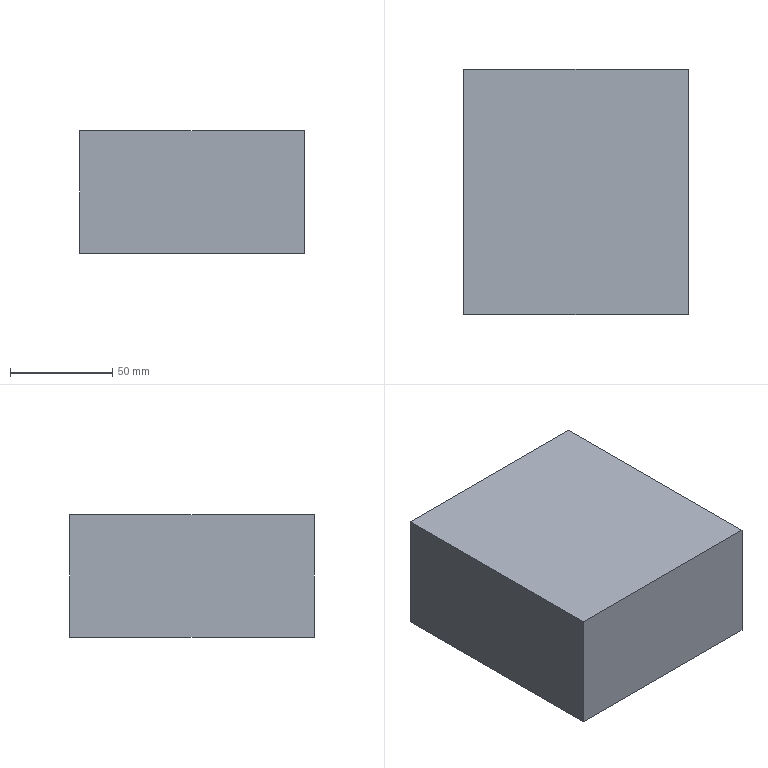Part | SolidWorks | features Extrusion 1, HoleWzd 1, PLine 1 | 1 solid | 15 faces | box 110 x 120 x 60 mm | volume 791822 mm3 | plane 7 | cylinder 4 | cone 4 | commonest cylinder face diameters 3.3 x4
STEP:
#1=CARTESIAN_POINT('',(1.65,15.,-19.9));
#2=VERTEX_POINT('',#1);
#3=CARTESIAN_POINT('',(-1.65,15.,-19.9));
#4=VERTEX_POINT('',#3);
#5=CARTESIAN_POINT('',(0.,15.,-19.9));
#6=DIRECTION('',(0.,0.,-1.));
#7=DIRECTION('',(-1.,0.,0.));
#8=AXIS2_PLACEMENT_3D('',#5,#6,#7);
#9=CIRCLE('',#8,1.65);
#10=EDGE_CURVE('',#2,#4,#9,.T.);
#11=ORIENTED_EDGE('',*,*,#10,.F.);
#12=CARTESIAN_POINT('',(1.65,15.,-30.));
#13=VERTEX_POINT('',#12);
#14=CARTESIAN_POINT('',(1.65,15.,-30.));
#15=DIRECTION('',(0.,0.,-1.));
#16=VECTOR('',#15,1000.);
#17=LINE('',#14,#16);
#18=EDGE_CURVE('',#2,#13,#17,.T.);
#19=ORIENTED_EDGE('',*,*,#18,.T.);
#20=CARTESIAN_POINT('',(-1.65,15.,-30.));
#21=VERTEX_POINT('',#20);
#22=CARTESIAN_POINT('',(0.,15.,-30.));
#23=DIRECTION('',(0.,0.,-1.));
#24=DIRECTION('',(-1.,0.,0.));
#25=AXIS2_PLACEMENT_3D('',#22,#23,#24);
#26=CIRCLE('',#25,1.65);
#27=EDGE_CURVE('',#13,#21,#26,.T.);
#28=ORIENTED_EDGE('',*,*,#27,.T.);
#29=CARTESIAN_POINT('',(-1.65,15.,-30.));
#30=DIRECTION('',(0.,0.,-1.));
#31=VECTOR('',#30,1000.);
#32=LINE('',#29,#31);
#33=EDGE_CURVE('',#4,#21,#32,.T.);
#34=ORIENTED_EDGE('',*,*,#33,.F.);
#35=EDGE_LOOP('',(#11,#19,#28,#34));
#36=FACE_OUTER_BOUND('',#35,.T.);
#37=CARTESIAN_POINT('',(0.,15.,-30.));
#38=DIRECTION('',(0.,0.,-1.));
#39=DIRECTION('',(-1.,0.,0.));
#40=AXIS2_PLACEMENT_3D('',#37,#38,#39);
#41=CYLINDRICAL_SURFACE('',#40,1.65);
#42=ADVANCED_FACE('',(#36),#41,.F.);
#43=CARTESIAN_POINT('',(0.,15.,-18.909));
#44=VERTEX_POINT('',#43);
#45=CARTESIAN_POINT('',(-1.65,15.,-19.9));
#46=DIRECTION('',(-0.8572,0.,-0.515));
#47=VECTOR('',#46,1000.);
#48=LINE('',#45,#47);
#49=EDGE_CURVE('',#44,#4,#48,.T.);
#50=ORIENTED_EDGE('',*,*,#49,.F.);
#51=CARTESIAN_POINT('',(1.65,15.,-19.9));
#52=DIRECTION('',(0.8572,0.,-0.515));
#53=VECTOR('',#52,1000.);
#54=LINE('',#51,#53);
#55=EDGE_CURVE('',#44,#2,#54,.T.);
#56=ORIENTED_EDGE('',*,*,#55,.T.);
#57=ORIENTED_EDGE('',*,*,#10,.T.);
#58=EDGE_LOOP('',(#50,#56,#57));
#59=FACE_OUTER_BOUND('',#58,.T.);
#60=CARTESIAN_POINT('',(0.,15.,-19.9));
#61=DIRECTION('',(0.,0.,-1.));
#62=DIRECTION('',(-1.,0.,0.));
#63=AXIS2_PLACEMENT_3D('',#60,#61,#62);
#64=CONICAL_SURFACE('',#63,1.65,1.03);
#65=ADVANCED_FACE('',(#59),#64,.F.);
#66=CARTESIAN_POINT('',(1.65,-15.,-19.9));
#67=VERTEX_POINT('',#66);
#68=CARTESIAN_POINT('',(-1.65,-15.,-19.9));
#69=VERTEX_POINT('',#68);
#70=CARTESIAN_POINT('',(0.,-15.,-19.9));
#71=DIRECTION('',(0.,0.,-1.));
#72=DIRECTION('',(-1.,0.,0.));
#73=AXIS2_PLACEMENT_3D('',#70,#71,#72);
#74=CIRCLE('',#73,1.65);
#75=EDGE_CURVE('',#67,#69,#74,.T.);
#76=ORIENTED_EDGE('',*,*,#75,.F.);
#77=CARTESIAN_POINT('',(1.65,-15.,-30.));
#78=VERTEX_POINT('',#77);
#79=CARTESIAN_POINT('',(1.65,-15.,-30.));
#80=DIRECTION('',(0.,0.,-1.));
#81=VECTOR('',#80,1000.);
#82=LINE('',#79,#81);
#83=EDGE_CURVE('',#67,#78,#82,.T.);
#84=ORIENTED_EDGE('',*,*,#83,.T.);
#85=CARTESIAN_POINT('',(-1.65,-15.,-30.));
#86=VERTEX_POINT('',#85);
#87=CARTESIAN_POINT('',(0.,-15.,-30.));
#88=DIRECTION('',(0.,0.,-1.));
#89=DIRECTION('',(-1.,0.,0.));
#90=AXIS2_PLACEMENT_3D('',#87,#88,#89);
#91=CIRCLE('',#90,1.65);
#92=EDGE_CURVE('',#78,#86,#91,.T.);
#93=ORIENTED_EDGE('',*,*,#92,.T.);
#94=CARTESIAN_POINT('',(-1.65,-15.,-30.));
#95=DIRECTION('',(0.,0.,-1.));
#96=VECTOR('',#95,1000.);
#97=LINE('',#94,#96);
#98=EDGE_CURVE('',#69,#86,#97,.T.);
#99=ORIENTED_EDGE('',*,*,#98,.F.);
#100=EDGE_LOOP('',(#76,#84,#93,#99));
#101=FACE_OUTER_BOUND('',#100,.T.);
#102=CARTESIAN_POINT('',(0.,-15.,-30.));
#103=DIRECTION('',(0.,0.,-1.));
#104=DIRECTION('',(-1.,0.,0.));
#105=AXIS2_PLACEMENT_3D('',#102,#103,#104);
#106=CYLINDRICAL_SURFACE('',#105,1.65);
#107=ADVANCED_FACE('',(#101),#106,.F.);
#108=CARTESIAN_POINT('',(0.,-15.,-18.909));
#109=VERTEX_POINT('',#108);
#110=CARTESIAN_POINT('',(-1.65,-15.,-19.9));
#111=DIRECTION('',(-0.8572,0.,-0.515));
#112=VECTOR('',#111,1000.);
#113=LINE('',#110,#112);
#114=EDGE_CURVE('',#109,#69,#113,.T.);
#115=ORIENTED_EDGE('',*,*,#114,.F.);
#116=CARTESIAN_POINT('',(1.65,-15.,-19.9));
#117=DIRECTION('',(0.8572,0.,-0.515));
#118=VECTOR('',#117,1000.);
#119=LINE('',#116,#118);
#120=EDGE_CURVE('',#109,#67,#119,.T.);
#121=ORIENTED_EDGE('',*,*,#120,.T.);
#122=ORIENTED_EDGE('',*,*,#75,.T.);
#123=EDGE_LOOP('',(#115,#121,#122));
#124=FACE_OUTER_BOUND('',#123,.T.);
#125=CARTESIAN_POINT('',(0.,-15.,-19.9));
#126=DIRECTION('',(0.,0.,-1.));
#127=DIRECTION('',(-1.,0.,0.));
#128=AXIS2_PLACEMENT_3D('',#125,#126,#127);
#129=CONICAL_SURFACE('',#128,1.65,1.03);
#130=ADVANCED_FACE('',(#124),#129,.F.);
#131=CARTESIAN_POINT('',(55.,-60.,-30.));
#132=VERTEX_POINT('',#131);
#133=CARTESIAN_POINT('',(55.,60.,-30.));
#134=VERTEX_POINT('',#133);
#135=CARTESIAN_POINT('',(55.,-60.,-30.));
#136=DIRECTION('',(0.,1.,0.));
#137=VECTOR('',#136,1000.);
#138=LINE('',#135,#137);
#139=EDGE_CURVE('',#132,#134,#138,.T.);
#140=ORIENTED_EDGE('',*,*,#139,.T.);
#141=CARTESIAN_POINT('',(55.,60.,30.));
#142=VERTEX_POINT('',#141);
#143=CARTESIAN_POINT('',(55.,60.,30.));
#144=DIRECTION('',(0.,0.,-1.));
#145=VECTOR('',#144,1000.);
#146=LINE('',#143,#145);
#147=EDGE_CURVE('',#142,#134,#146,.T.);
#148=ORIENTED_EDGE('',*,*,#147,.F.);
#149=CARTESIAN_POINT('',(55.,-60.,30.));
#150=VERTEX_POINT('',#149);
#151=CARTESIAN_POINT('',(55.,-60.,30.));
#152=DIRECTION('',(0.,1.,0.));
#153=VECTOR('',#152,1000.);
#154=LINE('',#151,#153);
#155=EDGE_CURVE('',#150,#142,#154,.T.);
#156=ORIENTED_EDGE('',*,*,#155,.F.);
#157=CARTESIAN_POINT('',(55.,-60.,30.));
#158=DIRECTION('',(0.,0.,-1.));
#159=VECTOR('',#158,1000.);
#160=LINE('',#157,#159);
#161=EDGE_CURVE('',#150,#132,#160,.T.);
#162=ORIENTED_EDGE('',*,*,#161,.T.);
#163=EDGE_LOOP('',(#140,#148,#156,#162));
#164=FACE_OUTER_BOUND('',#163,.T.);
#165=CARTESIAN_POINT('',(55.,-40.,-13.));
#166=VERTEX_POINT('',#165);
#167=CARTESIAN_POINT('',(55.,50.,-13.));
#168=VERTEX_POINT('',#167);
#169=CARTESIAN_POINT('',(55.,-60.,-13.));
#170=DIRECTION('',(0.,1.,0.));
#171=VECTOR('',#170,1000.);
#172=LINE('',#169,#171);
#173=EDGE_CURVE('',#166,#168,#172,.T.);
#174=ORIENTED_EDGE('',*,*,#173,.F.);
#175=CARTESIAN_POINT('',(55.,-40.,27.));
#176=VERTEX_POINT('',#175);
#177=CARTESIAN_POINT('',(55.,-40.,30.));
#178=DIRECTION('',(0.,0.,-1.));
#179=VECTOR('',#178,1000.);
#180=LINE('',#177,#179);
#181=EDGE_CURVE('',#176,#166,#180,.T.);
#182=ORIENTED_EDGE('',*,*,#181,.F.);
#183=CARTESIAN_POINT('',(55.,50.,27.));
#184=VERTEX_POINT('',#183);
#185=CARTESIAN_POINT('',(55.,-60.,27.));
#186=DIRECTION('',(0.,-1.,0.));
#187=VECTOR('',#186,1000.);
#188=LINE('',#185,#187);
#189=EDGE_CURVE('',#184,#176,#188,.T.);
#190=ORIENTED_EDGE('',*,*,#189,.F.);
#191=CARTESIAN_POINT('',(55.,50.,30.));
#192=DIRECTION('',(0.,0.,1.));
#193=VECTOR('',#192,1000.);
#194=LINE('',#191,#193);
#195=EDGE_CURVE('',#168,#184,#194,.T.);
#196=ORIENTED_EDGE('',*,*,#195,.F.);
#197=EDGE_LOOP('',(#174,#182,#190,#196));
#198=FACE_BOUND('',#197,.T.);
#199=CARTESIAN_POINT('',(55.,-60.,30.));
#200=DIRECTION('',(-1.,0.,0.));
#201=DIRECTION('',(0.,0.,1.));
#202=AXIS2_PLACEMENT_3D('',#199,#200,#201);
#203=PLANE('',#202);
#204=ADVANCED_FACE('',(#164,#198),#203,.F.);
#205=ORIENTED_EDGE('',*,*,#181,.T.);
#206=ORIENTED_EDGE('',*,*,#173,.T.);
#207=ORIENTED_EDGE('',*,*,#195,.T.);
#208=ORIENTED_EDGE('',*,*,#189,.T.);
#209=EDGE_LOOP('',(#205,#206,#207,#208));
#210=FACE_OUTER_BOUND('',#209,.T.);
#211=CARTESIAN_POINT('',(55.,-60.,30.));
#212=DIRECTION('',(-1.,0.,0.));
#213=DIRECTION('',(0.,0.,1.));
#214=AXIS2_PLACEMENT_3D('',#211,#212,#213);
#215=PLANE('',#214);
#216=ADVANCED_FACE('',(#210),#215,.F.);
#217=CARTESIAN_POINT('',(-55.,60.,-30.));
#218=VERTEX_POINT('',#217);
#219=CARTESIAN_POINT('',(-55.,60.,-30.));
#220=DIRECTION('',(-1.,0.,0.));
#221=VECTOR('',#220,1000.);
#222=LINE('',#219,#221);
#223=EDGE_CURVE('',#134,#218,#222,.T.);
#224=ORIENTED_EDGE('',*,*,#223,.T.);
#225=CARTESIAN_POINT('',(-55.,60.,30.));
#226=VERTEX_POINT('',#225);
#227=CARTESIAN_POINT('',(-55.,60.,30.));
#228=DIRECTION('',(0.,0.,-1.));
#229=VECTOR('',#228,1000.);
#230=LINE('',#227,#229);
#231=EDGE_CURVE('',#226,#218,#230,.T.);
#232=ORIENTED_EDGE('',*,*,#231,.F.);
#233=CARTESIAN_POINT('',(-55.,60.,30.));
#234=DIRECTION('',(-1.,0.,0.));
#235=VECTOR('',#234,1000.);
#236=LINE('',#233,#235);
#237=EDGE_CURVE('',#142,#226,#236,.T.);
#238=ORIENTED_EDGE('',*,*,#237,.F.);
#239=ORIENTED_EDGE('',*,*,#147,.T.);
#240=EDGE_LOOP('',(#224,#232,#238,#239));
#241=FACE_OUTER_BOUND('',#240,.T.);
#242=CARTESIAN_POINT('',(-55.,60.,30.));
#243=DIRECTION('',(0.,-1.,0.));
#244=DIRECTION('',(0.,0.,-1.));
#245=AXIS2_PLACEMENT_3D('',#242,#243,#244);
#246=PLANE('',#245);
#247=ADVANCED_FACE('',(#241),#246,.F.);
#248=CARTESIAN_POINT('',(-55.,-60.,-30.));
#249=VERTEX_POINT('',#248);
#250=CARTESIAN_POINT('',(-55.,-60.,-30.));
#251=DIRECTION('',(0.,-1.,0.));
#252=VECTOR('',#251,1000.);
#253=LINE('',#250,#252);
#254=EDGE_CURVE('',#218,#249,#253,.T.);
#255=ORIENTED_EDGE('',*,*,#254,.T.);
#256=CARTESIAN_POINT('',(-55.,-60.,30.));
#257=VERTEX_POINT('',#256);
#258=CARTESIAN_POINT('',(-55.,-60.,30.));
#259=DIRECTION('',(0.,0.,-1.));
#260=VECTOR('',#259,1000.);
#261=LINE('',#258,#260);
#262=EDGE_CURVE('',#257,#249,#261,.T.);
#263=ORIENTED_EDGE('',*,*,#262,.F.);
#264=CARTESIAN_POINT('',(-55.,-60.,30.));
#265=DIRECTION('',(0.,-1.,0.));
#266=VECTOR('',#265,1000.);
#267=LINE('',#264,#266);
#268=EDGE_CURVE('',#226,#257,#267,.T.);
#269=ORIENTED_EDGE('',*,*,#268,.F.);
#270=ORIENTED_EDGE('',*,*,#231,.T.);
#271=EDGE_LOOP('',(#255,#263,#269,#270));
#272=FACE_OUTER_BOUND('',#271,.T.);
#273=CARTESIAN_POINT('',(-55.,-60.,30.));
#274=DIRECTION('',(1.,0.,0.));
#275=DIRECTION('',(0.,0.,-1.));
#276=AXIS2_PLACEMENT_3D('',#273,#274,#275);
#277=PLANE('',#276);
#278=ADVANCED_FACE('',(#272),#277,.F.);
#279=CARTESIAN_POINT('',(-55.,-60.,-30.));
#280=DIRECTION('',(1.,0.,0.));
#281=VECTOR('',#280,1000.);
#282=LINE('',#279,#281);
#283=EDGE_CURVE('',#249,#132,#282,.T.);
#284=ORIENTED_EDGE('',*,*,#283,.T.);
#285=ORIENTED_EDGE('',*,*,#161,.F.);
#286=CARTESIAN_POINT('',(-55.,-60.,30.));
#287=DIRECTION('',(1.,0.,0.));
#288=VECTOR('',#287,1000.);
#289=LINE('',#286,#288);
#290=EDGE_CURVE('',#257,#150,#289,.T.);
#291=ORIENTED_EDGE('',*,*,#290,.F.);
#292=ORIENTED_EDGE('',*,*,#262,.T.);
#293=EDGE_LOOP('',(#284,#285,#291,#292));
#294=FACE_OUTER_BOUND('',#293,.T.);
#295=CARTESIAN_POINT('',(-55.,-60.,30.));
#296=DIRECTION('',(0.,1.,0.));
#297=DIRECTION('',(0.,0.,1.));
#298=AXIS2_PLACEMENT_3D('',#295,#296,#297);
#299=PLANE('',#298);
#300=ADVANCED_FACE('',(#294),#299,.F.);
#301=ORIENTED_EDGE('',*,*,#155,.T.);
#302=ORIENTED_EDGE('',*,*,#237,.T.);
#303=ORIENTED_EDGE('',*,*,#268,.T.);
#304=ORIENTED_EDGE('',*,*,#290,.T.);
#305=EDGE_LOOP('',(#301,#302,#303,#304));
#306=FACE_OUTER_BOUND('',#305,.T.);
#307=CARTESIAN_POINT('',(0.,0.,30.));
#308=DIRECTION('',(0.,0.,-1.));
#309=DIRECTION('',(-1.,0.,0.));
#310=AXIS2_PLACEMENT_3D('',#307,#308,#309);
#311=PLANE('',#310);
#312=ADVANCED_FACE('',(#306),#311,.F.);
#313=CARTESIAN_POINT('',(0.,15.,-30.));
#314=DIRECTION('',(0.,0.,-1.));
#315=DIRECTION('',(-1.,0.,0.));
#316=AXIS2_PLACEMENT_3D('',#313,#314,#315);
#317=CIRCLE('',#316,1.65);
#318=EDGE_CURVE('',#21,#13,#317,.T.);
#319=ORIENTED_EDGE('',*,*,#318,.F.);
#320=ORIENTED_EDGE('',*,*,#27,.F.);
#321=EDGE_LOOP('',(#319,#320));
#322=FACE_BOUND('',#321,.T.);
#323=CARTESIAN_POINT('',(0.,-15.,-30.));
#324=DIRECTION('',(0.,0.,-1.));
#325=DIRECTION('',(-1.,0.,0.));
#326=AXIS2_PLACEMENT_3D('',#323,#324,#325);
#327=CIRCLE('',#326,1.65);
#328=EDGE_CURVE('',#86,#78,#327,.T.);
#329=ORIENTED_EDGE('',*,*,#328,.F.);
#330=ORIENTED_EDGE('',*,*,#92,.F.);
#331=EDGE_LOOP('',(#329,#330));
#332=FACE_BOUND('',#331,.T.);
#333=ORIENTED_EDGE('',*,*,#139,.F.);
#334=ORIENTED_EDGE('',*,*,#283,.F.);
#335=ORIENTED_EDGE('',*,*,#254,.F.);
#336=ORIENTED_EDGE('',*,*,#223,.F.);
#337=EDGE_LOOP('',(#333,#334,#335,#336));
#338=FACE_OUTER_BOUND('',#337,.T.);
#339=CARTESIAN_POINT('',(0.,0.,-30.));
#340=DIRECTION('',(0.,0.,-1.));
#341=DIRECTION('',(-1.,0.,0.));
#342=AXIS2_PLACEMENT_3D('',#339,#340,#341);
#343=PLANE('',#342);
#344=ADVANCED_FACE('',(#322,#332,#338),#343,.T.);
#345=ORIENTED_EDGE('',*,*,#120,.F.);
#346=ORIENTED_EDGE('',*,*,#114,.T.);
#347=CARTESIAN_POINT('',(0.,-15.,-19.9));
#348=DIRECTION('',(0.,0.,-1.));
#349=DIRECTION('',(-1.,0.,0.));
#350=AXIS2_PLACEMENT_3D('',#347,#348,#349);
#351=CIRCLE('',#350,1.65);
#352=EDGE_CURVE('',#69,#67,#351,.T.);
#353=ORIENTED_EDGE('',*,*,#352,.T.);
#354=EDGE_LOOP('',(#345,#346,#353));
#355=FACE_OUTER_BOUND('',#354,.T.);
#356=CARTESIAN_POINT('',(0.,-15.,-19.9));
#357=DIRECTION('',(0.,0.,-1.));
#358=DIRECTION('',(-1.,0.,0.));
#359=AXIS2_PLACEMENT_3D('',#356,#357,#358);
#360=CONICAL_SURFACE('',#359,1.65,1.03);
#361=ADVANCED_FACE('',(#355),#360,.F.);
#362=ORIENTED_EDGE('',*,*,#83,.F.);
#363=ORIENTED_EDGE('',*,*,#352,.F.);
#364=ORIENTED_EDGE('',*,*,#98,.T.);
#365=ORIENTED_EDGE('',*,*,#328,.T.);
#366=EDGE_LOOP('',(#362,#363,#364,#365));
#367=FACE_OUTER_BOUND('',#366,.T.);
#368=CARTESIAN_POINT('',(0.,-15.,-30.));
#369=DIRECTION('',(0.,0.,-1.));
#370=DIRECTION('',(-1.,0.,0.));
#371=AXIS2_PLACEMENT_3D('',#368,#369,#370);
#372=CYLINDRICAL_SURFACE('',#371,1.65);
#373=ADVANCED_FACE('',(#367),#372,.F.);
#374=ORIENTED_EDGE('',*,*,#55,.F.);
#375=ORIENTED_EDGE('',*,*,#49,.T.);
#376=CARTESIAN_POINT('',(0.,15.,-19.9));
#377=DIRECTION('',(0.,0.,-1.));
#378=DIRECTION('',(-1.,0.,0.));
#379=AXIS2_PLACEMENT_3D('',#376,#377,#378);
#380=CIRCLE('',#379,1.65);
#381=EDGE_CURVE('',#4,#2,#380,.T.);
#382=ORIENTED_EDGE('',*,*,#381,.T.);
#383=EDGE_LOOP('',(#374,#375,#382));
#384=FACE_OUTER_BOUND('',#383,.T.);
#385=CARTESIAN_POINT('',(0.,15.,-19.9));
#386=DIRECTION('',(0.,0.,-1.));
#387=DIRECTION('',(-1.,0.,0.));
#388=AXIS2_PLACEMENT_3D('',#385,#386,#387);
#389=CONICAL_SURFACE('',#388,1.65,1.03);
#390=ADVANCED_FACE('',(#384),#389,.F.);
#391=ORIENTED_EDGE('',*,*,#18,.F.);
#392=ORIENTED_EDGE('',*,*,#381,.F.);
#393=ORIENTED_EDGE('',*,*,#33,.T.);
#394=ORIENTED_EDGE('',*,*,#318,.T.);
#395=EDGE_LOOP('',(#391,#392,#393,#394));
#396=FACE_OUTER_BOUND('',#395,.T.);
#397=CARTESIAN_POINT('',(0.,15.,-30.));
#398=DIRECTION('',(0.,0.,-1.));
#399=DIRECTION('',(-1.,0.,0.));
#400=AXIS2_PLACEMENT_3D('',#397,#398,#399);
#401=CYLINDRICAL_SURFACE('',#400,1.65);
#402=ADVANCED_FACE('',(#396),#401,.F.);
#403=CLOSED_SHELL('',(#42,#65,#107,#130,#204,#216,#247,#278,#300,#312,#344,#361,#373,#390,#402));
#404=MANIFOLD_SOLID_BREP('',#403);
#405=CARTESIAN_POINT('',(0.,0.,0.));
#406=DIRECTION('',(0.,0.,1.));
#407=DIRECTION('',(1.,0.,0.));
#408=AXIS2_PLACEMENT_3D('',#405,#406,#407);
#409=(LENGTH_UNIT()NAMED_UNIT(*)SI_UNIT(.MILLI.,.METRE.));
#410=UNCERTAINTY_MEASURE_WITH_UNIT(LENGTH_MEASURE(0.00001),#409,'','');
#411=(NAMED_UNIT(*)PLANE_ANGLE_UNIT()SI_UNIT($,.RADIAN.));
#412=(NAMED_UNIT(*)SI_UNIT($,.STERADIAN.)SOLID_ANGLE_UNIT());
#413=(GEOMETRIC_REPRESENTATION_CONTEXT(3)GLOBAL_UNCERTAINTY_ASSIGNED_CONTEXT((#410))GLOBAL_UNIT_ASSIGNED_CONTEXT((#409,#411,#412))REPRESENTATION_CONTEXT('',''));
#414=ADVANCED_BREP_SHAPE_REPRESENTATION('',(#404,#408),#413);